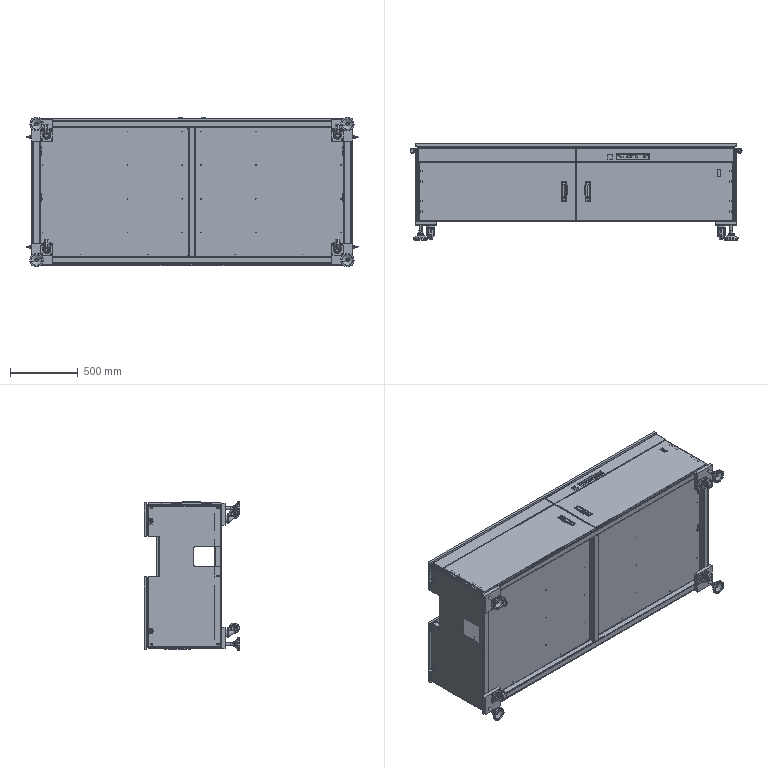Part | NX | features BREP 72 | 96 solids | 3753 faces | volume 54998715 mm3 | plane 1728 | cylinder 1639 | cone 156 | torus 120 | spline 84 | sphere 26 | commonest cylinder face diameters 3.3 x268 10 x127 5 x104 8 x104 7 x96 6 x78